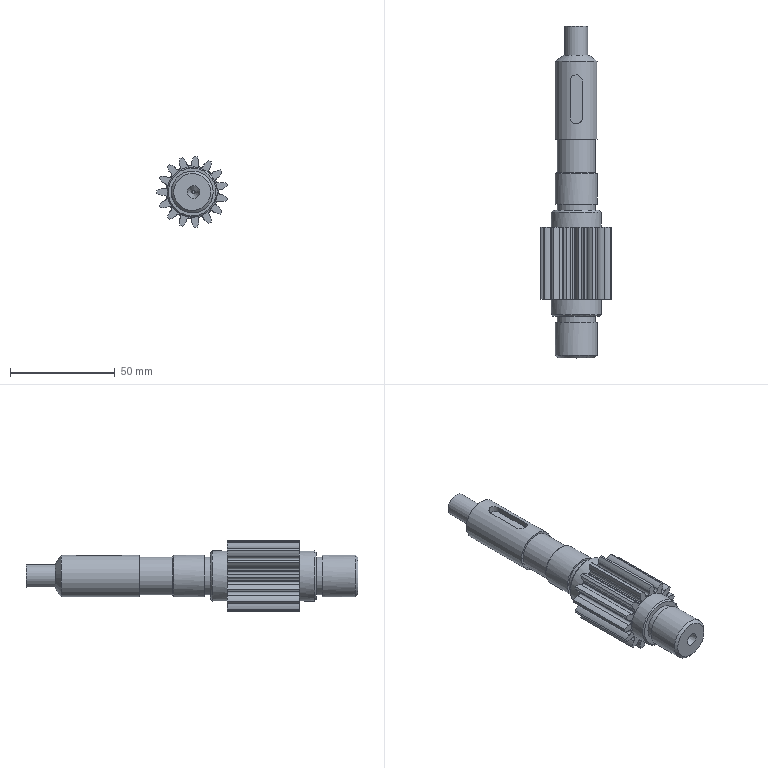Part | NX | features BREP 15, META 15, DATUM_CSYS 11, SKETCH 10, EXTRUDE 8, CHAMFER 4, DATUM_PLANE 2, HOLE PACKAGE 2, TAPER_HOLE 2, CYLINDER 1, FSET 1, RECT_SLOT 1, Resize Face 1, SWP104 1, SYMBOLIC_THREAD 1 | 10 solids | 133 faces | box 33.753 x 158.547 x 33.926 mm | volume 59659 mm3 | spline 75 | cylinder 26 | plane 25 | cone 7 | commonest cylinder face diameters 25 x15 18 x3 20 x3 5.9 x2 24 x2 11 x1